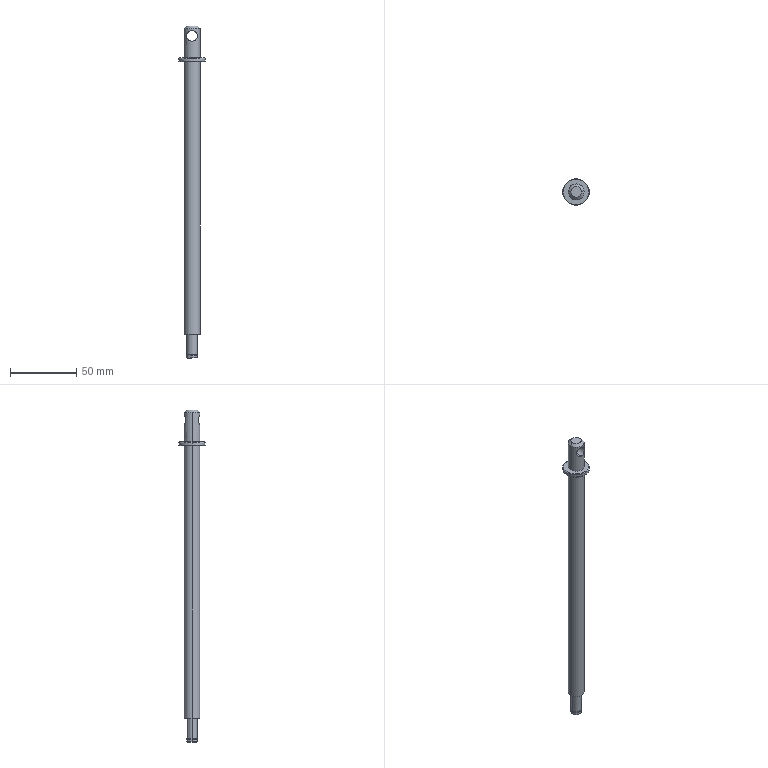Part | SolidWorks | features Chamfer 3, ICE 2, Revolution 1 | 1 solid | 29 faces | box 20 x 20 x 250 mm | volume 27080 mm3 | cylinder 14 | cone 8 | plane 7 | commonest cylinder face diameters 8 x6 12 x4 6.4 x2 20 x2
STEP:
#1=CARTESIAN_POINT('',(9.5,0.,432.269));
#2=VERTEX_POINT('',#1);
#3=CARTESIAN_POINT('',(-9.5,0.,432.269));
#4=VERTEX_POINT('',#3);
#5=CARTESIAN_POINT('',(0.,0.,432.269));
#6=DIRECTION('',(0.,0.,1.));
#7=DIRECTION('',(1.,0.,0.));
#8=AXIS2_PLACEMENT_3D('',#5,#6,#7);
#9=CIRCLE('',#8,9.5);
#10=EDGE_CURVE('',#2,#4,#9,.T.);
#11=ORIENTED_EDGE('',*,*,#10,.F.);
#12=CARTESIAN_POINT('',(10.,0.,431.769));
#13=VERTEX_POINT('',#12);
#14=CARTESIAN_POINT('',(9.5,0.,432.269));
#15=DIRECTION('',(0.7071,0.,-0.7071));
#16=VECTOR('',#15,1000.);
#17=LINE('',#14,#16);
#18=EDGE_CURVE('',#2,#13,#17,.T.);
#19=ORIENTED_EDGE('',*,*,#18,.T.);
#20=CARTESIAN_POINT('',(-10.,0.,431.769));
#21=VERTEX_POINT('',#20);
#22=CARTESIAN_POINT('',(0.,0.,431.769));
#23=DIRECTION('',(0.,0.,-1.));
#24=DIRECTION('',(1.,0.,0.));
#25=AXIS2_PLACEMENT_3D('',#22,#23,#24);
#26=CIRCLE('',#25,10.);
#27=EDGE_CURVE('',#21,#13,#26,.T.);
#28=ORIENTED_EDGE('',*,*,#27,.F.);
#29=CARTESIAN_POINT('',(-9.5,0.,432.269));
#30=DIRECTION('',(-0.7071,0.,-0.7071));
#31=VECTOR('',#30,1000.);
#32=LINE('',#29,#31);
#33=EDGE_CURVE('',#4,#21,#32,.T.);
#34=ORIENTED_EDGE('',*,*,#33,.F.);
#35=EDGE_LOOP('',(#11,#19,#28,#34));
#36=FACE_OUTER_BOUND('',#35,.T.);
#37=CARTESIAN_POINT('',(0.,0.,432.269));
#38=DIRECTION('',(0.,0.,-1.));
#39=DIRECTION('',(-1.,0.,0.));
#40=AXIS2_PLACEMENT_3D('',#37,#38,#39);
#41=CONICAL_SURFACE('',#40,9.5,0.7854);
#42=ADVANCED_FACE('',(#36),#41,.T.);
#43=CARTESIAN_POINT('',(-9.5,0.,429.269));
#44=VERTEX_POINT('',#43);
#45=CARTESIAN_POINT('',(9.5,0.,429.269));
#46=VERTEX_POINT('',#45);
#47=CARTESIAN_POINT('',(0.,0.,429.269));
#48=DIRECTION('',(0.,0.,-1.));
#49=DIRECTION('',(1.,0.,0.));
#50=AXIS2_PLACEMENT_3D('',#47,#48,#49);
#51=CIRCLE('',#50,9.5);
#52=EDGE_CURVE('',#44,#46,#51,.T.);
#53=ORIENTED_EDGE('',*,*,#52,.F.);
#54=CARTESIAN_POINT('',(-10.,0.,429.769));
#55=VERTEX_POINT('',#54);
#56=CARTESIAN_POINT('',(-10.,0.,429.769));
#57=DIRECTION('',(-0.7071,0.,0.7071));
#58=VECTOR('',#57,1000.);
#59=LINE('',#56,#58);
#60=EDGE_CURVE('',#44,#55,#59,.T.);
#61=ORIENTED_EDGE('',*,*,#60,.T.);
#62=CARTESIAN_POINT('',(10.,0.,429.769));
#63=VERTEX_POINT('',#62);
#64=CARTESIAN_POINT('',(0.,0.,429.769));
#65=DIRECTION('',(0.,0.,1.));
#66=DIRECTION('',(1.,0.,0.));
#67=AXIS2_PLACEMENT_3D('',#64,#65,#66);
#68=CIRCLE('',#67,10.);
#69=EDGE_CURVE('',#63,#55,#68,.T.);
#70=ORIENTED_EDGE('',*,*,#69,.F.);
#71=CARTESIAN_POINT('',(10.,0.,429.769));
#72=DIRECTION('',(0.7071,0.,0.7071));
#73=VECTOR('',#72,1000.);
#74=LINE('',#71,#73);
#75=EDGE_CURVE('',#46,#63,#74,.T.);
#76=ORIENTED_EDGE('',*,*,#75,.F.);
#77=EDGE_LOOP('',(#53,#61,#70,#76));
#78=FACE_OUTER_BOUND('',#77,.T.);
#79=CARTESIAN_POINT('',(0.,0.,429.769));
#80=DIRECTION('',(0.,0.,1.));
#81=DIRECTION('',(1.,0.,0.));
#82=AXIS2_PLACEMENT_3D('',#79,#80,#81);
#83=CONICAL_SURFACE('',#82,10.,0.7854);
#84=ADVANCED_FACE('',(#78),#83,.T.);
#85=CARTESIAN_POINT('',(0.,5.998,452.894));
#86=VERTEX_POINT('',#85);
#87=CARTESIAN_POINT('',(0.,5.998,444.894));
#88=VERTEX_POINT('',#87);
#89=CARTESIAN_POINT('',(0.,5.998,452.894));
#90=CARTESIAN_POINT('',(-0.2752,5.992,452.894));
#91=CARTESIAN_POINT('',(-0.5439,5.967,452.866));
#92=CARTESIAN_POINT('',(-1.069,5.882,452.758));
#93=CARTESIAN_POINT('',(-1.328,5.823,452.677));
#94=CARTESIAN_POINT('',(-1.81,5.679,452.471));
#95=CARTESIAN_POINT('',(-2.038,5.595,452.346));
#96=CARTESIAN_POINT('',(-2.465,5.409,452.055));
#97=CARTESIAN_POINT('',(-2.659,5.31,451.893));
#98=CARTESIAN_POINT('',(-3.015,5.106,451.535));
#99=CARTESIAN_POINT('',(-3.177,5.001,451.338));
#100=CARTESIAN_POINT('',(-3.459,4.802,450.919));
#101=CARTESIAN_POINT('',(-3.58,4.707,450.696));
#102=CARTESIAN_POINT('',(-3.782,4.54,450.221));
#103=CARTESIAN_POINT('',(-3.863,4.468,449.965));
#104=CARTESIAN_POINT('',(-3.944,4.393,449.572));
#105=CARTESIAN_POINT('',(-3.965,4.374,449.439));
#106=CARTESIAN_POINT('',(-3.993,4.347,449.168));
#107=CARTESIAN_POINT('',(-4.,4.34,449.03));
#108=CARTESIAN_POINT('',(-4.,4.341,448.62));
#109=CARTESIAN_POINT('',(-3.972,4.368,448.351));
#110=CARTESIAN_POINT('',(-3.863,4.468,447.821));
#111=CARTESIAN_POINT('',(-3.783,4.539,447.57));
#112=CARTESIAN_POINT('',(-3.581,4.706,447.094));
#113=CARTESIAN_POINT('',(-3.457,4.804,446.866));
#114=CARTESIAN_POINT('',(-3.174,5.003,446.447));
#115=CARTESIAN_POINT('',(-3.015,5.106,446.253));
#116=CARTESIAN_POINT('',(-2.659,5.31,445.895));
#117=CARTESIAN_POINT('',(-2.461,5.411,445.731));
#118=CARTESIAN_POINT('',(-2.04,5.594,445.444));
#119=CARTESIAN_POINT('',(-1.814,5.677,445.32));
#120=CARTESIAN_POINT('',(-1.331,5.822,445.113));
#121=CARTESIAN_POINT('',(-1.073,5.882,445.032));
#122=CARTESIAN_POINT('',(-0.6789,5.945,444.95));
#123=CARTESIAN_POINT('',(-0.5455,5.962,444.929));
#124=CARTESIAN_POINT('',(-0.2747,5.987,444.901));
#125=CARTESIAN_POINT('',(-0.1365,5.995,444.894));
#126=CARTESIAN_POINT('',(0.,5.998,444.894));
#127=B_SPLINE_CURVE_WITH_KNOTS('',3,(#89,#90,#91,#92,#93,#94,#95,#96,#97,#98,#99,#100,#101,#102,#103,#104,#105,#106,#107,#108,#109,#110,#111,#112,#113,#114,#115,#116,#117,#118,#119,#120,#121,#122,#123,#124,#125,#126),.UNSPECIFIED.,.F.,.F.,(4,2,2,2,2,2,2,2,2,2,2,2,2,2,2,2,2,2,4),(0.,0.0008127,0.001625,0.002438,0.003251,0.004064,0.004876,0.005689,0.006095,0.006502,0.007314,0.008127,0.00894,0.009752,0.01057,0.01138,0.01219,0.0126,0.013),.UNSPECIFIED.);
#128=EDGE_CURVE('',#86,#88,#127,.T.);
#129=ORIENTED_EDGE('',*,*,#128,.T.);
#130=CARTESIAN_POINT('',(0.,5.998,444.894));
#131=CARTESIAN_POINT('',(0.2698,6.005,444.894));
#132=CARTESIAN_POINT('',(0.5365,5.993,444.921));
#133=CARTESIAN_POINT('',(1.064,5.935,445.029));
#134=CARTESIAN_POINT('',(1.32,5.889,445.109));
#135=CARTESIAN_POINT('',(1.804,5.771,445.314));
#136=CARTESIAN_POINT('',(2.035,5.698,445.441));
#137=CARTESIAN_POINT('',(2.461,5.538,445.731));
#138=CARTESIAN_POINT('',(2.657,5.451,445.894));
#139=CARTESIAN_POINT('',(3.018,5.27,446.256));
#140=CARTESIAN_POINT('',(3.179,5.178,446.453));
#141=CARTESIAN_POINT('',(3.461,5.001,446.874));
#142=CARTESIAN_POINT('',(3.584,4.916,447.1));
#143=CARTESIAN_POINT('',(3.787,4.768,447.58));
#144=CARTESIAN_POINT('',(3.865,4.706,447.83));
#145=CARTESIAN_POINT('',(3.945,4.641,448.222));
#146=CARTESIAN_POINT('',(3.966,4.624,448.356));
#147=CARTESIAN_POINT('',(3.993,4.601,448.624));
#148=CARTESIAN_POINT('',(4.007,4.59,448.892));
#149=CARTESIAN_POINT('',(3.993,4.601,449.16));
#150=CARTESIAN_POINT('',(3.967,4.623,449.427));
#151=CARTESIAN_POINT('',(3.946,4.64,449.562));
#152=CARTESIAN_POINT('',(3.866,4.705,449.955));
#153=CARTESIAN_POINT('',(3.788,4.767,450.205));
#154=CARTESIAN_POINT('',(3.585,4.916,450.687));
#155=CARTESIAN_POINT('',(3.463,5.,450.912));
#156=CARTESIAN_POINT('',(3.18,5.177,451.333));
#157=CARTESIAN_POINT('',(3.019,5.269,451.531));
#158=CARTESIAN_POINT('',(2.659,5.45,451.893));
#159=CARTESIAN_POINT('',(2.464,5.537,452.056));
#160=CARTESIAN_POINT('',(2.041,5.696,452.344));
#161=CARTESIAN_POINT('',(1.809,5.769,452.471));
#162=CARTESIAN_POINT('',(1.325,5.888,452.678));
#163=CARTESIAN_POINT('',(1.072,5.933,452.757));
#164=CARTESIAN_POINT('',(0.5444,5.992,452.866));
#165=CARTESIAN_POINT('',(0.272,6.005,452.894));
#166=CARTESIAN_POINT('',(0.,5.998,452.894));
#167=B_SPLINE_CURVE_WITH_KNOTS('',3,(#130,#131,#132,#133,#134,#135,#136,#137,#138,#139,#140,#141,#142,#143,#144,#145,#146,#147,#148,#149,#150,#151,#152,#153,#154,#155,#156,#157,#158,#159,#160,#161,#162,#163,#164,#165,#166),.UNSPECIFIED.,.F.,.F.,(4,2,2,2,2,2,2,2,2,1,2,2,2,2,2,2,2,2,4),(0.013,0.01381,0.01461,0.01541,0.01622,0.01702,0.01782,0.01863,0.01903,0.01943,0.01983,0.02023,0.02103,0.02184,0.02264,0.02344,0.02425,0.02505,0.02585),.UNSPECIFIED.);
#168=EDGE_CURVE('',#88,#86,#167,.T.);
#169=ORIENTED_EDGE('',*,*,#168,.T.);
#170=EDGE_LOOP('',(#129,#169));
#171=FACE_BOUND('',#170,.T.);
#172=CARTESIAN_POINT('',(-5.858,0.,454.269));
#173=VERTEX_POINT('',#172);
#174=CARTESIAN_POINT('',(6.142,0.,454.269));
#175=VERTEX_POINT('',#174);
#176=CARTESIAN_POINT('',(0.1424,0.,454.269));
#177=DIRECTION('',(0.,0.,-1.));
#178=DIRECTION('',(-1.,0.,0.));
#179=AXIS2_PLACEMENT_3D('',#176,#177,#178);
#180=CIRCLE('',#179,6.);
#181=EDGE_CURVE('',#173,#175,#180,.T.);
#182=ORIENTED_EDGE('',*,*,#181,.T.);
#183=CARTESIAN_POINT('',(6.142,0.,432.269));
#184=VERTEX_POINT('',#183);
#185=CARTESIAN_POINT('',(6.142,0.,206.269));
#186=DIRECTION('',(0.,0.,-1.));
#187=VECTOR('',#186,1000.);
#188=LINE('',#185,#187);
#189=EDGE_CURVE('',#175,#184,#188,.T.);
#190=ORIENTED_EDGE('',*,*,#189,.T.);
#191=CARTESIAN_POINT('',(-5.858,0.,432.269));
#192=VERTEX_POINT('',#191);
#193=CARTESIAN_POINT('',(0.1424,0.,432.269));
#194=DIRECTION('',(0.,0.,1.));
#195=DIRECTION('',(1.,0.,0.));
#196=AXIS2_PLACEMENT_3D('',#193,#194,#195);
#197=CIRCLE('',#196,6.);
#198=EDGE_CURVE('',#184,#192,#197,.T.);
#199=ORIENTED_EDGE('',*,*,#198,.T.);
#200=CARTESIAN_POINT('',(-5.858,0.,206.269));
#201=DIRECTION('',(0.,0.,-1.));
#202=VECTOR('',#201,1000.);
#203=LINE('',#200,#202);
#204=EDGE_CURVE('',#173,#192,#203,.T.);
#205=ORIENTED_EDGE('',*,*,#204,.F.);
#206=EDGE_LOOP('',(#182,#190,#199,#205));
#207=FACE_OUTER_BOUND('',#206,.T.);
#208=CARTESIAN_POINT('',(0.1424,0.,206.269));
#209=DIRECTION('',(0.,0.,-1.));
#210=DIRECTION('',(-1.,0.,0.));
#211=AXIS2_PLACEMENT_3D('',#208,#209,#210);
#212=CYLINDRICAL_SURFACE('',#211,6.);
#213=ADVANCED_FACE('',(#171,#207),#212,.T.);
#214=CARTESIAN_POINT('',(4.142,0.,456.269));
#215=VERTEX_POINT('',#214);
#216=CARTESIAN_POINT('',(-3.858,0.,456.269));
#217=VERTEX_POINT('',#216);
#218=CARTESIAN_POINT('',(0.1424,0.,456.269));
#219=DIRECTION('',(0.,0.,1.));
#220=DIRECTION('',(-1.,0.,0.));
#221=AXIS2_PLACEMENT_3D('',#218,#219,#220);
#222=CIRCLE('',#221,4.);
#223=EDGE_CURVE('',#215,#217,#222,.T.);
#224=ORIENTED_EDGE('',*,*,#223,.F.);
#225=CARTESIAN_POINT('',(6.142,0.,454.269));
#226=DIRECTION('',(0.7071,0.,-0.7071));
#227=VECTOR('',#226,1000.);
#228=LINE('',#225,#227);
#229=EDGE_CURVE('',#215,#175,#228,.T.);
#230=ORIENTED_EDGE('',*,*,#229,.T.);
#231=ORIENTED_EDGE('',*,*,#181,.F.);
#232=CARTESIAN_POINT('',(-5.858,0.,454.269));
#233=DIRECTION('',(-0.7071,0.,-0.7071));
#234=VECTOR('',#233,1000.);
#235=LINE('',#232,#234);
#236=EDGE_CURVE('',#217,#173,#235,.T.);
#237=ORIENTED_EDGE('',*,*,#236,.F.);
#238=EDGE_LOOP('',(#224,#230,#231,#237));
#239=FACE_OUTER_BOUND('',#238,.T.);
#240=CARTESIAN_POINT('',(0.1424,0.,454.269));
#241=DIRECTION('',(0.,0.,-1.));
#242=DIRECTION('',(-1.,0.,0.));
#243=AXIS2_PLACEMENT_3D('',#240,#241,#242);
#244=CONICAL_SURFACE('',#243,6.,0.7854);
#245=ADVANCED_FACE('',(#239),#244,.T.);
#246=CARTESIAN_POINT('',(0.,-5.998,444.894));
#247=VERTEX_POINT('',#246);
#248=CARTESIAN_POINT('',(0.,-5.998,452.894));
#249=VERTEX_POINT('',#248);
#250=CARTESIAN_POINT('',(0.,-5.998,444.894));
#251=CARTESIAN_POINT('',(-0.1354,-5.995,444.894));
#252=CARTESIAN_POINT('',(-0.2706,-5.987,444.901));
#253=CARTESIAN_POINT('',(-0.5409,-5.963,444.929));
#254=CARTESIAN_POINT('',(-0.6765,-5.945,444.95));
#255=CARTESIAN_POINT('',(-1.073,-5.882,445.031));
#256=CARTESIAN_POINT('',(-1.326,-5.823,445.111));
#257=CARTESIAN_POINT('',(-1.812,-5.678,445.318));
#258=CARTESIAN_POINT('',(-2.04,-5.594,445.444));
#259=CARTESIAN_POINT('',(-2.463,-5.41,445.732));
#260=CARTESIAN_POINT('',(-2.661,-5.309,445.897));
#261=CARTESIAN_POINT('',(-3.017,-5.105,446.255));
#262=CARTESIAN_POINT('',(-3.176,-5.002,446.449));
#263=CARTESIAN_POINT('',(-3.459,-4.802,446.87));
#264=CARTESIAN_POINT('',(-3.583,-4.705,447.097));
#265=CARTESIAN_POINT('',(-3.784,-4.538,447.573));
#266=CARTESIAN_POINT('',(-3.864,-4.467,447.826));
#267=CARTESIAN_POINT('',(-3.972,-4.367,448.354));
#268=CARTESIAN_POINT('',(-4.,-4.34,448.623));
#269=CARTESIAN_POINT('',(-4.,-4.341,449.172));
#270=CARTESIAN_POINT('',(-3.971,-4.368,449.443));
#271=CARTESIAN_POINT('',(-3.863,-4.468,449.968));
#272=CARTESIAN_POINT('',(-3.782,-4.541,450.223));
#273=CARTESIAN_POINT('',(-3.58,-4.708,450.698));
#274=CARTESIAN_POINT('',(-3.457,-4.804,450.923));
#275=CARTESIAN_POINT('',(-3.172,-5.005,451.345));
#276=CARTESIAN_POINT('',(-3.012,-5.108,451.539));
#277=CARTESIAN_POINT('',(-2.655,-5.312,451.896));
#278=CARTESIAN_POINT('',(-2.457,-5.412,452.061));
#279=CARTESIAN_POINT('',(-2.035,-5.596,452.348));
#280=CARTESIAN_POINT('',(-1.81,-5.679,452.471));
#281=CARTESIAN_POINT('',(-1.329,-5.822,452.676));
#282=CARTESIAN_POINT('',(-1.07,-5.882,452.758));
#283=CARTESIAN_POINT('',(-0.5443,-5.966,452.866));
#284=CARTESIAN_POINT('',(-0.2747,-5.992,452.894));
#285=CARTESIAN_POINT('',(0.,-5.998,452.894));
#286=B_SPLINE_CURVE_WITH_KNOTS('',3,(#250,#251,#252,#253,#254,#255,#256,#257,#258,#259,#260,#261,#262,#263,#264,#265,#266,#267,#268,#269,#270,#271,#272,#273,#274,#275,#276,#277,#278,#279,#280,#281,#282,#283,#284,#285),.UNSPECIFIED.,.F.,.F.,(4,2,2,2,2,2,2,2,2,2,2,2,2,2,2,2,2,4),(0.01287,0.01328,0.01368,0.01449,0.01531,0.01612,0.01693,0.01774,0.01855,0.01936,0.02017,0.02099,0.0218,0.02261,0.02342,0.02423,0.02504,0.02585),.UNSPECIFIED.);
#287=EDGE_CURVE('',#247,#249,#286,.T.);
#288=ORIENTED_EDGE('',*,*,#287,.F.);
#289=CARTESIAN_POINT('',(0.,-25.,444.894));
#290=DIRECTION('',(0.,1.,0.));
#291=VECTOR('',#290,1000.);
#292=LINE('',#289,#291);
#293=EDGE_CURVE('',#247,#88,#292,.T.);
#294=ORIENTED_EDGE('',*,*,#293,.T.);
#295=ORIENTED_EDGE('',*,*,#128,.F.);
#296=CARTESIAN_POINT('',(0.,-25.,452.894));
#297=DIRECTION('',(0.,1.,0.));
#298=VECTOR('',#297,1000.);
#299=LINE('',#296,#298);
#300=EDGE_CURVE('',#249,#86,#299,.T.);
#301=ORIENTED_EDGE('',*,*,#300,.F.);
#302=EDGE_LOOP('',(#288,#294,#295,#301));
#303=FACE_OUTER_BOUND('',#302,.T.);
#304=CARTESIAN_POINT('',(0.,-25.,448.894));
#305=DIRECTION('',(0.,1.,0.));
#306=DIRECTION('',(0.,0.,1.));
#307=AXIS2_PLACEMENT_3D('',#304,#305,#306);
#308=CYLINDRICAL_SURFACE('',#307,4.);
#309=ADVANCED_FACE('',(#303),#308,.F.);
#310=ORIENTED_EDGE('',*,*,#27,.T.);
#311=CARTESIAN_POINT('',(10.,0.,432.269));
#312=DIRECTION('',(0.,0.,-1.));
#313=VECTOR('',#312,1000.);
#314=LINE('',#311,#313);
#315=EDGE_CURVE('',#13,#63,#314,.T.);
#316=ORIENTED_EDGE('',*,*,#315,.T.);
#317=ORIENTED_EDGE('',*,*,#69,.T.);
#318=CARTESIAN_POINT('',(-10.,0.,432.269));
#319=DIRECTION('',(0.,0.,-1.));
#320=VECTOR('',#319,1000.);
#321=LINE('',#318,#320);
#322=EDGE_CURVE('',#21,#55,#321,.T.);
#323=ORIENTED_EDGE('',*,*,#322,.F.);
#324=EDGE_LOOP('',(#310,#316,#317,#323));
#325=FACE_OUTER_BOUND('',#324,.T.);
#326=CARTESIAN_POINT('',(0.,0.,432.269));
#327=DIRECTION('',(0.,0.,-1.));
#328=DIRECTION('',(-1.,0.,0.));
#329=AXIS2_PLACEMENT_3D('',#326,#327,#328);
#330=CYLINDRICAL_SURFACE('',#329,10.);
#331=ADVANCED_FACE('',(#325),#330,.T.);
#332=CARTESIAN_POINT('',(-3.658,0.,206.269));
#333=VERTEX_POINT('',#332);
#334=CARTESIAN_POINT('',(3.942,0.,206.269));
#335=VERTEX_POINT('',#334);
#336=CARTESIAN_POINT('',(0.1424,0.,206.269));
#337=DIRECTION('',(0.,0.,-1.));
#338=DIRECTION('',(1.,0.,0.));
#339=AXIS2_PLACEMENT_3D('',#336,#337,#338);
#340=CIRCLE('',#339,3.8);
#341=EDGE_CURVE('',#333,#335,#340,.T.);
#342=ORIENTED_EDGE('',*,*,#341,.F.);
#343=CARTESIAN_POINT('',(-3.858,0.,206.469));
#344=VERTEX_POINT('',#343);
#345=CARTESIAN_POINT('',(-3.658,0.,206.269));
#346=DIRECTION('',(-0.7071,0.,0.7071));
#347=VECTOR('',#346,1000.);
#348=LINE('',#345,#347);
#349=EDGE_CURVE('',#333,#344,#348,.T.);
#350=ORIENTED_EDGE('',*,*,#349,.T.);
#351=CARTESIAN_POINT('',(4.142,0.,206.469));
#352=VERTEX_POINT('',#351);
#353=CARTESIAN_POINT('',(0.1424,0.,206.469));
#354=DIRECTION('',(0.,0.,1.));
#355=DIRECTION('',(1.,0.,0.));
#356=AXIS2_PLACEMENT_3D('',#353,#354,#355);
#357=CIRCLE('',#356,4.);
#358=EDGE_CURVE('',#352,#344,#357,.T.);
#359=ORIENTED_EDGE('',*,*,#358,.F.);
#360=CARTESIAN_POINT('',(3.942,0.,206.269));
#361=DIRECTION('',(0.7071,0.,0.7071));
#362=VECTOR('',#361,1000.);
#363=LINE('',#360,#362);
#364=EDGE_CURVE('',#335,#352,#363,.T.);
#365=ORIENTED_EDGE('',*,*,#364,.F.);
#366=EDGE_LOOP('',(#342,#350,#359,#365));
#367=FACE_OUTER_BOUND('',#366,.T.);
#368=CARTESIAN_POINT('',(0.1424,0.,206.269));
#369=DIRECTION('',(0.,0.,1.));
#370=DIRECTION('',(1.,0.,0.));
#371=AXIS2_PLACEMENT_3D('',#368,#369,#370);
#372=CONICAL_SURFACE('',#371,3.8,0.7854);
#373=ADVANCED_FACE('',(#367),#372,.T.);
#374=CARTESIAN_POINT('',(-3.858,0.,208.269));
#375=VERTEX_POINT('',#374);
#376=CARTESIAN_POINT('',(4.142,0.,208.269));
#377=VERTEX_POINT('',#376);
#378=CARTESIAN_POINT('',(0.1424,0.,208.269));
#379=DIRECTION('',(0.,0.,-1.));
#380=DIRECTION('',(-1.,0.,0.));
#381=AXIS2_PLACEMENT_3D('',#378,#379,#380);
#382=CIRCLE('',#381,4.);
#383=EDGE_CURVE('',#375,#377,#382,.T.);
#384=ORIENTED_EDGE('',*,*,#383,.T.);
#385=CARTESIAN_POINT('',(4.142,0.,206.269));
#386=DIRECTION('',(0.,0.,-1.));
#387=VECTOR('',#386,1000.);
#388=LINE('',#385,#387);
#389=EDGE_CURVE('',#377,#352,#388,.T.);
#390=ORIENTED_EDGE('',*,*,#389,.T.);
#391=ORIENTED_EDGE('',*,*,#358,.T.);
#392=CARTESIAN_POINT('',(-3.858,0.,206.269));
#393=DIRECTION('',(0.,0.,-1.));
#394=VECTOR('',#393,1000.);
#395=LINE('',#392,#394);
#396=EDGE_CURVE('',#375,#344,#395,.T.);
#397=ORIENTED_EDGE('',*,*,#396,.F.);
#398=EDGE_LOOP('',(#384,#390,#391,#397));
#399=FACE_OUTER_BOUND('',#398,.T.);
#400=CARTESIAN_POINT('',(0.1424,0.,206.269));
#401=DIRECTION('',(0.,0.,-1.));
#402=DIRECTION('',(-1.,0.,0.));
#403=AXIS2_PLACEMENT_3D('',#400,#401,#402);
#404=CYLINDRICAL_SURFACE('',#403,4.);
#405=ADVANCED_FACE('',(#399),#404,.T.);
#406=CARTESIAN_POINT('',(-3.058,0.,209.169));
#407=VERTEX_POINT('',#406);
#408=CARTESIAN_POINT('',(3.342,0.,209.169));
#409=VERTEX_POINT('',#408);
#410=CARTESIAN_POINT('',(0.1424,0.,209.169));
#411=DIRECTION('',(0.,0.,-1.));
#412=DIRECTION('',(-1.,0.,0.));
#413=AXIS2_PLACEMENT_3D('',#410,#411,#412);
#414=CIRCLE('',#413,3.2);
#415=EDGE_CURVE('',#407,#409,#414,.T.);
#416=ORIENTED_EDGE('',*,*,#415,.T.);
#417=CARTESIAN_POINT('',(3.342,0.,208.269));
#418=VERTEX_POINT('',#417);
#419=CARTESIAN_POINT('',(3.342,0.,206.269));
#420=DIRECTION('',(0.,0.,-1.));
#421=VECTOR('',#420,1000.);
#422=LINE('',#419,#421);
#423=EDGE_CURVE('',#409,#418,#422,.T.);
#424=ORIENTED_EDGE('',*,*,#423,.T.);
#425=CARTESIAN_POINT('',(-3.058,0.,208.269));
#426=VERTEX_POINT('',#425);
#427=CARTESIAN_POINT('',(0.1424,0.,208.269));
#428=DIRECTION('',(0.,0.,-1.));
#429=DIRECTION('',(-1.,0.,0.));
#430=AXIS2_PLACEMENT_3D('',#427,#428,#429);
#431=CIRCLE('',#430,3.2);
#432=EDGE_CURVE('',#426,#418,#431,.T.);
#433=ORIENTED_EDGE('',*,*,#432,.F.);
#434=CARTESIAN_POINT('',(-3.058,0.,206.269));
#435=DIRECTION('',(0.,0.,-1.));
#436=VECTOR('',#435,1000.);
#437=LINE('',#434,#436);
#438=EDGE_CURVE('',#407,#426,#437,.T.);
#439=ORIENTED_EDGE('',*,*,#438,.F.);
#440=EDGE_LOOP('',(#416,#424,#433,#439));
#441=FACE_OUTER_BOUND('',#440,.T.);
#442=CARTESIAN_POINT('',(0.1424,0.,206.269));
#443=DIRECTION('',(0.,0.,-1.));
#444=DIRECTION('',(-1.,0.,0.));
#445=AXIS2_PLACEMENT_3D('',#442,#443,#444);
#446=CYLINDRICAL_SURFACE('',#445,3.2);
#447=ADVANCED_FACE('',(#441),#446,.T.);
#448=CARTESIAN_POINT('',(-3.858,0.,224.269));
#449=VERTEX_POINT('',#448);
#450=CARTESIAN_POINT('',(4.142,0.,224.269));
#451=VERTEX_POINT('',#450);
#452=CARTESIAN_POINT('',(0.1424,0.,224.269));
#453=DIRECTION('',(0.,0.,-1.));
#454=DIRECTION('',(-1.,0.,0.));
#455=AXIS2_PLACEMENT_3D('',#452,#453,#454);
#456=CIRCLE('',#455,4.);
#457=EDGE_CURVE('',#449,#451,#456,.T.);
#458=ORIENTED_EDGE('',*,*,#457,.T.);
#459=CARTESIAN_POINT('',(4.142,0.,209.169));
#460=VERTEX_POINT('',#459);
#461=CARTESIAN_POINT('',(4.142,0.,206.269));
#462=DIRECTION('',(0.,0.,-1.));
#463=VECTOR('',#462,1000.);
#464=LINE('',#461,#463);
#465=EDGE_CURVE('',#451,#460,#464,.T.);
#466=ORIENTED_EDGE('',*,*,#465,.T.);
#467=CARTESIAN_POINT('',(-3.858,0.,209.169));
#468=VERTEX_POINT('',#467);
#469=CARTESIAN_POINT('',(0.1424,0.,209.169));
#470=DIRECTION('',(0.,0.,-1.));
#471=DIRECTION('',(-1.,0.,0.));
#472=AXIS2_PLACEMENT_3D('',#469,#470,#471);
#473=CIRCLE('',#472,4.);
#474=EDGE_CURVE('',#468,#460,#473,.T.);
#475=ORIENTED_EDGE('',*,*,#474,.F.);
#476=CARTESIAN_POINT('',(-3.858,0.,206.269));
#477=DIRECTION('',(0.,0.,-1.));
#478=VECTOR('',#477,1000.);
#479=LINE('',#476,#478);
#480=EDGE_CURVE('',#449,#468,#479,.T.);
#481=ORIENTED_EDGE('',*,*,#480,.F.);
#482=EDGE_LOOP('',(#458,#466,#475,#481));
#483=FACE_OUTER_BOUND('',#482,.T.);
#484=CARTESIAN_POINT('',(0.1424,0.,206.269));
#485=DIRECTION('',(0.,0.,-1.));
#486=DIRECTION('',(-1.,0.,0.));
#487=AXIS2_PLACEMENT_3D('',#484,#485,#486);
#488=CYLINDRICAL_SURFACE('',#487,4.);
#489=ADVANCED_FACE('',(#483),#488,.T.);
#490=CARTESIAN_POINT('',(6.142,0.,429.269));
#491=VERTEX_POINT('',#490);
#492=CARTESIAN_POINT('',(-5.858,0.,429.269));
#493=VERTEX_POINT('',#492);
#494=CARTESIAN_POINT('',(0.1424,0.,429.269));
#495=DIRECTION('',(0.,0.,1.));
#496=DIRECTION('',(1.,0.,0.));
#497=AXIS2_PLACEMENT_3D('',#494,#495,#496);
#498=CIRCLE('',#497,6.);
#499=EDGE_CURVE('',#491,#493,#498,.T.);
#500=ORIENTED_EDGE('',*,*,#499,.F.);
#501=CARTESIAN_POINT('',(6.142,0.,224.269));
#502=VERTEX_POINT('',#501);
#503=CARTESIAN_POINT('',(6.142,0.,206.269));
#504=DIRECTION('',(0.,0.,-1.));
#505=VECTOR('',#504,1000.);
#506=LINE('',#503,#505);
#507=EDGE_CURVE('',#491,#502,#506,.T.);
#508=ORIENTED_EDGE('',*,*,#507,.T.);
#509=CARTESIAN_POINT('',(-5.858,0.,224.269));
#510=VERTEX_POINT('',#509);
#511=CARTESIAN_POINT('',(0.1424,0.,224.269));
#512=DIRECTION('',(0.,0.,-1.));
#513=DIRECTION('',(-1.,0.,0.));
#514=AXIS2_PLACEMENT_3D('',#511,#512,#513);
#515=CIRCLE('',#514,6.);
#516=EDGE_CURVE('',#510,#502,#515,.T.);
#517=ORIENTED_EDGE('',*,*,#516,.F.);
#518=CARTESIAN_POINT('',(-5.858,0.,206.269));
#519=DIRECTION('',(0.,0.,-1.));
#520=VECTOR('',#519,1000.);
#521=LINE('',#518,#520);
#522=EDGE_CURVE('',#493,#510,#521,.T.);
#523=ORIENTED_EDGE('',*,*,#522,.F.);
#524=EDGE_LOOP('',(#500,#508,#517,#523));
#525=FACE_OUTER_BOUND('',#524,.T.);
#526=CARTESIAN_POINT('',(0.1424,0.,206.269));
#527=DIRECTION('',(0.,0.,-1.));
#528=DIRECTION('',(-1.,0.,0.));
#529=AXIS2_PLACEMENT_3D('',#526,#527,#528);
#530=CYLINDRICAL_SURFACE('',#529,6.);
#531=ADVANCED_FACE('',(#525),#530,.T.);
#532=ORIENTED_EDGE('',*,*,#507,.F.);
#533=CARTESIAN_POINT('',(0.1424,0.,429.269));
#534=DIRECTION('',(0.,0.,1.));
#535=DIRECTION('',(1.,0.,0.));
#536=AXIS2_PLACEMENT_3D('',#533,#534,#535);
#537=CIRCLE('',#536,6.);
#538=EDGE_CURVE('',#493,#491,#537,.T.);
#539=ORIENTED_EDGE('',*,*,#538,.F.);
#540=ORIENTED_EDGE('',*,*,#522,.T.);
#541=CARTESIAN_POINT('',(0.1424,0.,224.269));
#542=DIRECTION('',(0.,0.,-1.));
#543=DIRECTION('',(-1.,0.,0.));
#544=AXIS2_PLACEMENT_3D('',#541,#542,#543);
#545=CIRCLE('',#544,6.);
#546=EDGE_CURVE('',#502,#510,#545,.T.);
#547=ORIENTED_EDGE('',*,*,#546,.F.);
#548=EDGE_LOOP('',(#532,#539,#540,#547));
#549=FACE_OUTER_BOUND('',#548,.T.);
#550=CARTESIAN_POINT('',(0.1424,0.,206.269));
#551=DIRECTION('',(0.,0.,-1.));
#552=DIRECTION('',(-1.,0.,0.));
#553=AXIS2_PLACEMENT_3D('',#550,#551,#552);
#554=CYLINDRICAL_SURFACE('',#553,6.);
#555=ADVANCED_FACE('',(#549),#554,.T.);
#556=ORIENTED_EDGE('',*,*,#457,.F.);
#557=CARTESIAN_POINT('',(0.1424,0.,224.269));
#558=DIRECTION('',(0.,0.,-1.));
#559=DIRECTION('',(-1.,0.,0.));
#560=AXIS2_PLACEMENT_3D('',#557,#558,#559);
#561=CIRCLE('',#560,4.);
#562=EDGE_CURVE('',#451,#449,#561,.T.);
#563=ORIENTED_EDGE('',*,*,#562,.F.);
#564=EDGE_LOOP('',(#556,#563));
#565=FACE_BOUND('',#564,.T.);
#566=ORIENTED_EDGE('',*,*,#516,.T.);
#567=ORIENTED_EDGE('',*,*,#546,.T.);
#568=EDGE_LOOP('',(#566,#567));
#569=FACE_OUTER_BOUND('',#568,.T.);
#570=CARTESIAN_POINT('',(6.142,0.,224.269));
#571=DIRECTION('',(0.,0.,1.));
#572=DIRECTION('',(1.,0.,0.));
#573=AXIS2_PLACEMENT_3D('',#570,#571,#572);
#574=PLANE('',#573);
#575=ADVANCED_FACE('',(#565,#569),#574,.F.);
#576=ORIENTED_EDGE('',*,*,#465,.F.);
#577=ORIENTED_EDGE('',*,*,#562,.T.);
#578=ORIENTED_EDGE('',*,*,#480,.T.);
#579=CARTESIAN_POINT('',(0.1424,0.,209.169));
#580=DIRECTION('',(0.,0.,-1.));
#581=DIRECTION('',(-1.,0.,0.));
#582=AXIS2_PLACEMENT_3D('',#579,#580,#581);
#583=CIRCLE('',#582,4.);
#584=EDGE_CURVE('',#460,#468,#583,.T.);
#585=ORIENTED_EDGE('',*,*,#584,.F.);
#586=EDGE_LOOP('',(#576,#577,#578,#585));
#587=FACE_OUTER_BOUND('',#586,.T.);
#588=CARTESIAN_POINT('',(0.1424,0.,206.269));
#589=DIRECTION('',(0.,0.,-1.));
#590=DIRECTION('',(-1.,0.,0.));
#591=AXIS2_PLACEMENT_3D('',#588,#589,#590);
#592=CYLINDRICAL_SURFACE('',#591,4.);
#593=ADVANCED_FACE('',(#587),#592,.T.);
#594=ORIENTED_EDGE('',*,*,#415,.F.);
#595=CARTESIAN_POINT('',(0.1424,0.,209.169));
#596=DIRECTION('',(0.,0.,-1.));
#597=DIRECTION('',(-1.,0.,0.));
#598=AXIS2_PLACEMENT_3D('',#595,#596,#597);
#599=CIRCLE('',#598,3.2);
#600=EDGE_CURVE('',#409,#407,#599,.T.);
#601=ORIENTED_EDGE('',*,*,#600,.F.);
#602=EDGE_LOOP('',(#594,#601));
#603=FACE_BOUND('',#602,.T.);
#604=ORIENTED_EDGE('',*,*,#474,.T.);
#605=ORIENTED_EDGE('',*,*,#584,.T.);
#606=EDGE_LOOP('',(#604,#605));
#607=FACE_OUTER_BOUND('',#606,.T.);
#608=CARTESIAN_POINT('',(3.342,0.,209.169));
#609=DIRECTION('',(0.,0.,1.));
#610=DIRECTION('',(1.,0.,0.));
#611=AXIS2_PLACEMENT_3D('',#608,#609,#610);
#612=PLANE('',#611);
#613=ADVANCED_FACE('',(#603,#607),#612,.F.);
#614=ORIENTED_EDGE('',*,*,#423,.F.);
#615=ORIENTED_EDGE('',*,*,#600,.T.);
#616=ORIENTED_EDGE('',*,*,#438,.T.);
#617=CARTESIAN_POINT('',(0.1424,0.,208.269));
#618=DIRECTION('',(0.,0.,-1.));
#619=DIRECTION('',(-1.,0.,0.));
#620=AXIS2_PLACEMENT_3D('',#617,#618,#619);
#621=CIRCLE('',#620,3.2);
#622=EDGE_CURVE('',#418,#426,#621,.T.);
#623=ORIENTED_EDGE('',*,*,#622,.F.);
#624=EDGE_LOOP('',(#614,#615,#616,#623));
#625=FACE_OUTER_BOUND('',#624,.T.);
#626=CARTESIAN_POINT('',(0.1424,0.,206.269));
#627=DIRECTION('',(0.,0.,-1.));
#628=DIRECTION('',(-1.,0.,0.));
#629=AXIS2_PLACEMENT_3D('',#626,#627,#628);
#630=CYLINDRICAL_SURFACE('',#629,3.2);
#631=ADVANCED_FACE('',(#625),#630,.T.);
#632=ORIENTED_EDGE('',*,*,#383,.F.);
#633=CARTESIAN_POINT('',(0.1424,0.,208.269));
#634=DIRECTION('',(0.,0.,-1.));
#635=DIRECTION('',(-1.,0.,0.));
#636=AXIS2_PLACEMENT_3D('',#633,#634,#635);
#637=CIRCLE('',#636,4.);
#638=EDGE_CURVE('',#377,#375,#637,.T.);
#639=ORIENTED_EDGE('',*,*,#638,.F.);
#640=EDGE_LOOP('',(#632,#639));
#641=FACE_OUTER_BOUND('',#640,.T.);
#642=ORIENTED_EDGE('',*,*,#432,.T.);
#643=ORIENTED_EDGE('',*,*,#622,.T.);
#644=EDGE_LOOP('',(#642,#643));
#645=FACE_BOUND('',#644,.T.);
#646=CARTESIAN_POINT('',(4.142,0.,208.269));
#647=DIRECTION('',(0.,0.,-1.));
#648=DIRECTION('',(-1.,0.,0.));
#649=AXIS2_PLACEMENT_3D('',#646,#647,#648);
#650=PLANE('',#649);
#651=ADVANCED_FACE('',(#641,#645),#650,.F.);
#652=ORIENTED_EDGE('',*,*,#389,.F.);
#653=ORIENTED_EDGE('',*,*,#638,.T.);
#654=ORIENTED_EDGE('',*,*,#396,.T.);
#655=CARTESIAN_POINT('',(0.1424,0.,206.469));
#656=DIRECTION('',(0.,0.,1.));
#657=DIRECTION('',(1.,0.,0.));
#658=AXIS2_PLACEMENT_3D('',#655,#656,#657);
#659=CIRCLE('',#658,4.);
#660=EDGE_CURVE('',#344,#352,#659,.T.);
#661=ORIENTED_EDGE('',*,*,#660,.T.);
#662=EDGE_LOOP('',(#652,#653,#654,#661));
#663=FACE_OUTER_BOUND('',#662,.T.);
#664=CARTESIAN_POINT('',(0.1424,0.,206.269));
#665=DIRECTION('',(0.,0.,-1.));
#666=DIRECTION('',(-1.,0.,0.));
#667=AXIS2_PLACEMENT_3D('',#664,#665,#666);
#668=CYLINDRICAL_SURFACE('',#667,4.);
#669=ADVANCED_FACE('',(#663),#668,.T.);
#670=CARTESIAN_POINT('',(0.1424,0.,206.269));
#671=DIRECTION('',(0.,0.,-1.));
#672=DIRECTION('',(1.,0.,0.));
#673=AXIS2_PLACEMENT_3D('',#670,#671,#672);
#674=CIRCLE('',#673,3.8);
#675=EDGE_CURVE('',#335,#333,#674,.T.);
#676=ORIENTED_EDGE('',*,*,#675,.T.);
#677=ORIENTED_EDGE('',*,*,#341,.T.);
#678=EDGE_LOOP('',(#676,#677));
#679=FACE_OUTER_BOUND('',#678,.T.);
#680=CARTESIAN_POINT('',(0.1424,0.,206.269));
#681=DIRECTION('',(0.,0.,1.));
#682=DIRECTION('',(1.,0.,0.));
#683=AXIS2_PLACEMENT_3D('',#680,#681,#682);
#684=PLANE('',#683);
#685=ADVANCED_FACE('',(#679),#684,.F.);
#686=ORIENTED_EDGE('',*,*,#349,.F.);
#687=ORIENTED_EDGE('',*,*,#675,.F.);
#688=ORIENTED_EDGE('',*,*,#364,.T.);
#689=ORIENTED_EDGE('',*,*,#660,.F.);
#690=EDGE_LOOP('',(#686,#687,#688,#689));
#691=FACE_OUTER_BOUND('',#690,.T.);
#692=CARTESIAN_POINT('',(0.1424,0.,206.269));
#693=DIRECTION('',(0.,0.,1.));
#694=DIRECTION('',(1.,0.,0.));
#695=AXIS2_PLACEMENT_3D('',#692,#693,#694);
#696=CONICAL_SURFACE('',#695,3.8,0.7854);
#697=ADVANCED_FACE('',(#691),#696,.T.);
#698=ORIENTED_EDGE('',*,*,#315,.F.);
#699=CARTESIAN_POINT('',(0.,0.,431.769));
#700=DIRECTION('',(0.,0.,-1.));
#701=DIRECTION('',(1.,0.,0.));
#702=AXIS2_PLACEMENT_3D('',#699,#700,#701);
#703=CIRCLE('',#702,10.);
#704=EDGE_CURVE('',#13,#21,#703,.T.);
#705=ORIENTED_EDGE('',*,*,#704,.T.);
#706=ORIENTED_EDGE('',*,*,#322,.T.);
#707=CARTESIAN_POINT('',(0.,0.,429.769));
#708=DIRECTION('',(0.,0.,1.));
#709=DIRECTION('',(1.,0.,0.));
#710=AXIS2_PLACEMENT_3D('',#707,#708,#709);
#711=CIRCLE('',#710,10.);
#712=EDGE_CURVE('',#55,#63,#711,.T.);
#713=ORIENTED_EDGE('',*,*,#712,.T.);
#714=EDGE_LOOP('',(#698,#705,#706,#713));
#715=FACE_OUTER_BOUND('',#714,.T.);
#716=CARTESIAN_POINT('',(0.,0.,432.269));
#717=DIRECTION('',(0.,0.,-1.));
#718=DIRECTION('',(-1.,0.,0.));
#719=AXIS2_PLACEMENT_3D('',#716,#717,#718);
#720=CYLINDRICAL_SURFACE('',#719,10.);
#721=ADVANCED_FACE('',(#715),#720,.T.);
#722=CARTESIAN_POINT('',(0.,0.,432.269));
#723=DIRECTION('',(0.,0.,1.));
#724=DIRECTION('',(1.,0.,0.));
#725=AXIS2_PLACEMENT_3D('',#722,#723,#724);
#726=CIRCLE('',#725,9.5);
#727=EDGE_CURVE('',#4,#2,#726,.T.);
#728=ORIENTED_EDGE('',*,*,#727,.T.);
#729=ORIENTED_EDGE('',*,*,#10,.T.);
#730=EDGE_LOOP('',(#728,#729));
#731=FACE_OUTER_BOUND('',#730,.T.);
#732=CARTESIAN_POINT('',(0.1424,0.,432.269));
#733=DIRECTION('',(0.,0.,1.));
#734=DIRECTION('',(1.,0.,0.));
#735=AXIS2_PLACEMENT_3D('',#732,#733,#734);
#736=CIRCLE('',#735,6.);
#737=EDGE_CURVE('',#192,#184,#736,.T.);
#738=ORIENTED_EDGE('',*,*,#737,.F.);
#739=ORIENTED_EDGE('',*,*,#198,.F.);
#740=EDGE_LOOP('',(#738,#739));
#741=FACE_BOUND('',#740,.T.);
#742=CARTESIAN_POINT('',(0.,0.,432.269));
#743=DIRECTION('',(0.,0.,1.));
#744=DIRECTION('',(1.,0.,0.));
#745=AXIS2_PLACEMENT_3D('',#742,#743,#744);
#746=PLANE('',#745);
#747=ADVANCED_FACE('',(#731,#741),#746,.T.);
#748=CARTESIAN_POINT('',(0.,0.,429.269));
#749=DIRECTION('',(0.,0.,-1.));
#750=DIRECTION('',(1.,0.,0.));
#751=AXIS2_PLACEMENT_3D('',#748,#749,#750);
#752=CIRCLE('',#751,9.5);
#753=EDGE_CURVE('',#46,#44,#752,.T.);
#754=ORIENTED_EDGE('',*,*,#753,.T.);
#755=ORIENTED_EDGE('',*,*,#52,.T.);
#756=EDGE_LOOP('',(#754,#755));
#757=FACE_OUTER_BOUND('',#756,.T.);
#758=ORIENTED_EDGE('',*,*,#538,.T.);
#759=ORIENTED_EDGE('',*,*,#499,.T.);
#760=EDGE_LOOP('',(#758,#759));
#761=FACE_BOUND('',#760,.T.);
#762=CARTESIAN_POINT('',(0.,0.,429.269));
#763=DIRECTION('',(0.,0.,1.));
#764=DIRECTION('',(1.,0.,0.));
#765=AXIS2_PLACEMENT_3D('',#762,#763,#764);
#766=PLANE('',#765);
#767=ADVANCED_FACE('',(#757,#761),#766,.F.);
#768=CARTESIAN_POINT('',(0.1424,0.,456.269));
#769=DIRECTION('',(0.,0.,1.));
#770=DIRECTION('',(-1.,0.,0.));
#771=AXIS2_PLACEMENT_3D('',#768,#769,#770);
#772=CIRCLE('',#771,4.);
#773=EDGE_CURVE('',#217,#215,#772,.T.);
#774=ORIENTED_EDGE('',*,*,#773,.T.);
#775=ORIENTED_EDGE('',*,*,#223,.T.);
#776=EDGE_LOOP('',(#774,#775));
#777=FACE_OUTER_BOUND('',#776,.T.);
#778=CARTESIAN_POINT('',(6.142,0.,456.269));
#779=DIRECTION('',(0.,0.,-1.));
#780=DIRECTION('',(-1.,0.,0.));
#781=AXIS2_PLACEMENT_3D('',#778,#779,#780);
#782=PLANE('',#781);
#783=ADVANCED_FACE('',(#777),#782,.F.);
#784=ORIENTED_EDGE('',*,*,#293,.F.);
#785=CARTESIAN_POINT('',(0.,-5.998,452.894));
#786=CARTESIAN_POINT('',(0.2724,-6.005,452.894));
#787=CARTESIAN_POINT('',(0.5392,-5.993,452.867));
#788=CARTESIAN_POINT('',(1.063,-5.935,452.76));
#789=CARTESIAN_POINT('',(1.321,-5.888,452.679));
#790=CARTESIAN_POINT('',(1.804,-5.771,452.474));
#791=CARTESIAN_POINT('',(2.033,-5.699,452.349));
#792=CARTESIAN_POINT('',(2.462,-5.538,452.057));
#793=CARTESIAN_POINT('',(2.658,-5.451,451.894));
#794=CARTESIAN_POINT('',(3.016,-5.271,451.534));
#795=CARTESIAN_POINT('',(3.179,-5.178,451.336));
#796=CARTESIAN_POINT('',(3.462,-5.001,450.914));
#797=CARTESIAN_POINT('',(3.583,-4.917,450.691));
#798=CARTESIAN_POINT('',(3.785,-4.769,450.214));
#799=CARTESIAN_POINT('',(3.865,-4.706,449.959));
#800=CARTESIAN_POINT('',(3.945,-4.641,449.569));
#801=CARTESIAN_POINT('',(3.965,-4.624,449.437));
#802=CARTESIAN_POINT('',(3.993,-4.602,449.169));
#803=CARTESIAN_POINT('',(4.,-4.596,449.032));
#804=CARTESIAN_POINT('',(4.,-4.595,448.627));
#805=CARTESIAN_POINT('',(3.973,-4.618,448.36));
#806=CARTESIAN_POINT('',(3.867,-4.705,447.835));
#807=CARTESIAN_POINT('',(3.788,-4.767,447.583));
#808=CARTESIAN_POINT('',(3.586,-4.915,447.104));
#809=CARTESIAN_POINT('',(3.462,-5.001,446.875));
#810=CARTESIAN_POINT('',(3.178,-5.178,446.453));
#811=CARTESIAN_POINT('',(3.017,-5.27,446.256));
#812=CARTESIAN_POINT('',(2.656,-5.452,445.893));
#813=CARTESIAN_POINT('',(2.461,-5.539,445.73));
#814=CARTESIAN_POINT('',(2.037,-5.697,445.442));
#815=CARTESIAN_POINT('',(1.807,-5.77,445.316));
#816=CARTESIAN_POINT('',(1.32,-5.889,445.109));
#817=CARTESIAN_POINT('',(1.068,-5.934,445.03));
#818=CARTESIAN_POINT('',(0.6726,-5.978,444.949));
#819=CARTESIAN_POINT('',(0.5375,-5.988,444.928));
#820=CARTESIAN_POINT('',(0.2686,-6.,444.901));
#821=CARTESIAN_POINT('',(0.1342,-6.001,444.894));
#822=CARTESIAN_POINT('',(0.,-5.998,444.894));
#823=B_SPLINE_CURVE_WITH_KNOTS('',3,(#785,#786,#787,#788,#789,#790,#791,#792,#793,#794,#795,#796,#797,#798,#799,#800,#801,#802,#803,#804,#805,#806,#807,#808,#809,#810,#811,#812,#813,#814,#815,#816,#817,#818,#819,#820,#821,#822),.UNSPECIFIED.,.F.,.F.,(4,2,2,2,2,2,2,2,2,2,2,2,2,2,2,2,2,2,4),(0.,0.0008045,0.001609,0.002413,0.003218,0.004022,0.004827,0.005631,0.006033,0.006436,0.00724,0.008045,0.008849,0.009653,0.01046,0.01126,0.01207,0.01247,0.01287),.UNSPECIFIED.);
#824=EDGE_CURVE('',#249,#247,#823,.T.);
#825=ORIENTED_EDGE('',*,*,#824,.F.);
#826=ORIENTED_EDGE('',*,*,#300,.T.);
#827=ORIENTED_EDGE('',*,*,#168,.F.);
#828=EDGE_LOOP('',(#784,#825,#826,#827));
#829=FACE_OUTER_BOUND('',#828,.T.);
#830=CARTESIAN_POINT('',(0.,-25.,448.894));
#831=DIRECTION('',(0.,1.,0.));
#832=DIRECTION('',(0.,0.,1.));
#833=AXIS2_PLACEMENT_3D('',#830,#831,#832);
#834=CYLINDRICAL_SURFACE('',#833,4.);
#835=ADVANCED_FACE('',(#829),#834,.F.);
#836=ORIENTED_EDGE('',*,*,#229,.F.);
#837=ORIENTED_EDGE('',*,*,#773,.F.);
#838=ORIENTED_EDGE('',*,*,#236,.T.);
#839=CARTESIAN_POINT('',(0.1424,0.,454.269));
#840=DIRECTION('',(0.,0.,-1.));
#841=DIRECTION('',(-1.,0.,0.));
#842=AXIS2_PLACEMENT_3D('',#839,#840,#841);
#843=CIRCLE('',#842,6.);
#844=EDGE_CURVE('',#175,#173,#843,.T.);
#845=ORIENTED_EDGE('',*,*,#844,.F.);
#846=EDGE_LOOP('',(#836,#837,#838,#845));
#847=FACE_OUTER_BOUND('',#846,.T.);
#848=CARTESIAN_POINT('',(0.1424,0.,454.269));
#849=DIRECTION('',(0.,0.,-1.));
#850=DIRECTION('',(-1.,0.,0.));
#851=AXIS2_PLACEMENT_3D('',#848,#849,#850);
#852=CONICAL_SURFACE('',#851,6.,0.7854);
#853=ADVANCED_FACE('',(#847),#852,.T.);
#854=ORIENTED_EDGE('',*,*,#189,.F.);
#855=ORIENTED_EDGE('',*,*,#844,.T.);
#856=ORIENTED_EDGE('',*,*,#204,.T.);
#857=ORIENTED_EDGE('',*,*,#737,.T.);
#858=EDGE_LOOP('',(#854,#855,#856,#857));
#859=FACE_OUTER_BOUND('',#858,.T.);
#860=ORIENTED_EDGE('',*,*,#824,.T.);
#861=ORIENTED_EDGE('',*,*,#287,.T.);
#862=EDGE_LOOP('',(#860,#861));
#863=FACE_BOUND('',#862,.T.);
#864=CARTESIAN_POINT('',(0.1424,0.,206.269));
#865=DIRECTION('',(0.,0.,-1.));
#866=DIRECTION('',(-1.,0.,0.));
#867=AXIS2_PLACEMENT_3D('',#864,#865,#866);
#868=CYLINDRICAL_SURFACE('',#867,6.);
#869=ADVANCED_FACE('',(#859,#863),#868,.T.);
#870=ORIENTED_EDGE('',*,*,#60,.F.);
#871=ORIENTED_EDGE('',*,*,#753,.F.);
#872=ORIENTED_EDGE('',*,*,#75,.T.);
#873=ORIENTED_EDGE('',*,*,#712,.F.);
#874=EDGE_LOOP('',(#870,#871,#872,#873));
#875=FACE_OUTER_BOUND('',#874,.T.);
#876=CARTESIAN_POINT('',(0.,0.,429.769));
#877=DIRECTION('',(0.,0.,1.));
#878=DIRECTION('',(1.,0.,0.));
#879=AXIS2_PLACEMENT_3D('',#876,#877,#878);
#880=CONICAL_SURFACE('',#879,10.,0.7854);
#881=ADVANCED_FACE('',(#875),#880,.T.);
#882=ORIENTED_EDGE('',*,*,#18,.F.);
#883=ORIENTED_EDGE('',*,*,#727,.F.);
#884=ORIENTED_EDGE('',*,*,#33,.T.);
#885=ORIENTED_EDGE('',*,*,#704,.F.);
#886=EDGE_LOOP('',(#882,#883,#884,#885));
#887=FACE_OUTER_BOUND('',#886,.T.);
#888=CARTESIAN_POINT('',(0.,0.,432.269));
#889=DIRECTION('',(0.,0.,-1.));
#890=DIRECTION('',(-1.,0.,0.));
#891=AXIS2_PLACEMENT_3D('',#888,#889,#890);
#892=CONICAL_SURFACE('',#891,9.5,0.7854);
#893=ADVANCED_FACE('',(#887),#892,.T.);
#894=CLOSED_SHELL('',(#42,#84,#213,#245,#309,#331,#373,#405,#447,#489,#531,#555,#575,#593,#613,#631,#651,#669,#685,#697,#721,#747,#767,#783,#835,#853,#869,#881,#893));
#895=MANIFOLD_SOLID_BREP('',#894);
#896=CARTESIAN_POINT('',(0.,0.,0.));
#897=DIRECTION('',(0.,0.,1.));
#898=DIRECTION('',(1.,0.,0.));
#899=AXIS2_PLACEMENT_3D('',#896,#897,#898);
#900=(LENGTH_UNIT()NAMED_UNIT(*)SI_UNIT(.MILLI.,.METRE.));
#901=UNCERTAINTY_MEASURE_WITH_UNIT(LENGTH_MEASURE(0.00001),#900,'','');
#902=(NAMED_UNIT(*)PLANE_ANGLE_UNIT()SI_UNIT($,.RADIAN.));
#903=(NAMED_UNIT(*)SI_UNIT($,.STERADIAN.)SOLID_ANGLE_UNIT());
#904=(GEOMETRIC_REPRESENTATION_CONTEXT(3)GLOBAL_UNCERTAINTY_ASSIGNED_CONTEXT((#901))GLOBAL_UNIT_ASSIGNED_CONTEXT((#900,#902,#903))REPRESENTATION_CONTEXT('',''));
#905=ADVANCED_BREP_SHAPE_REPRESENTATION('',(#895,#899),#904);